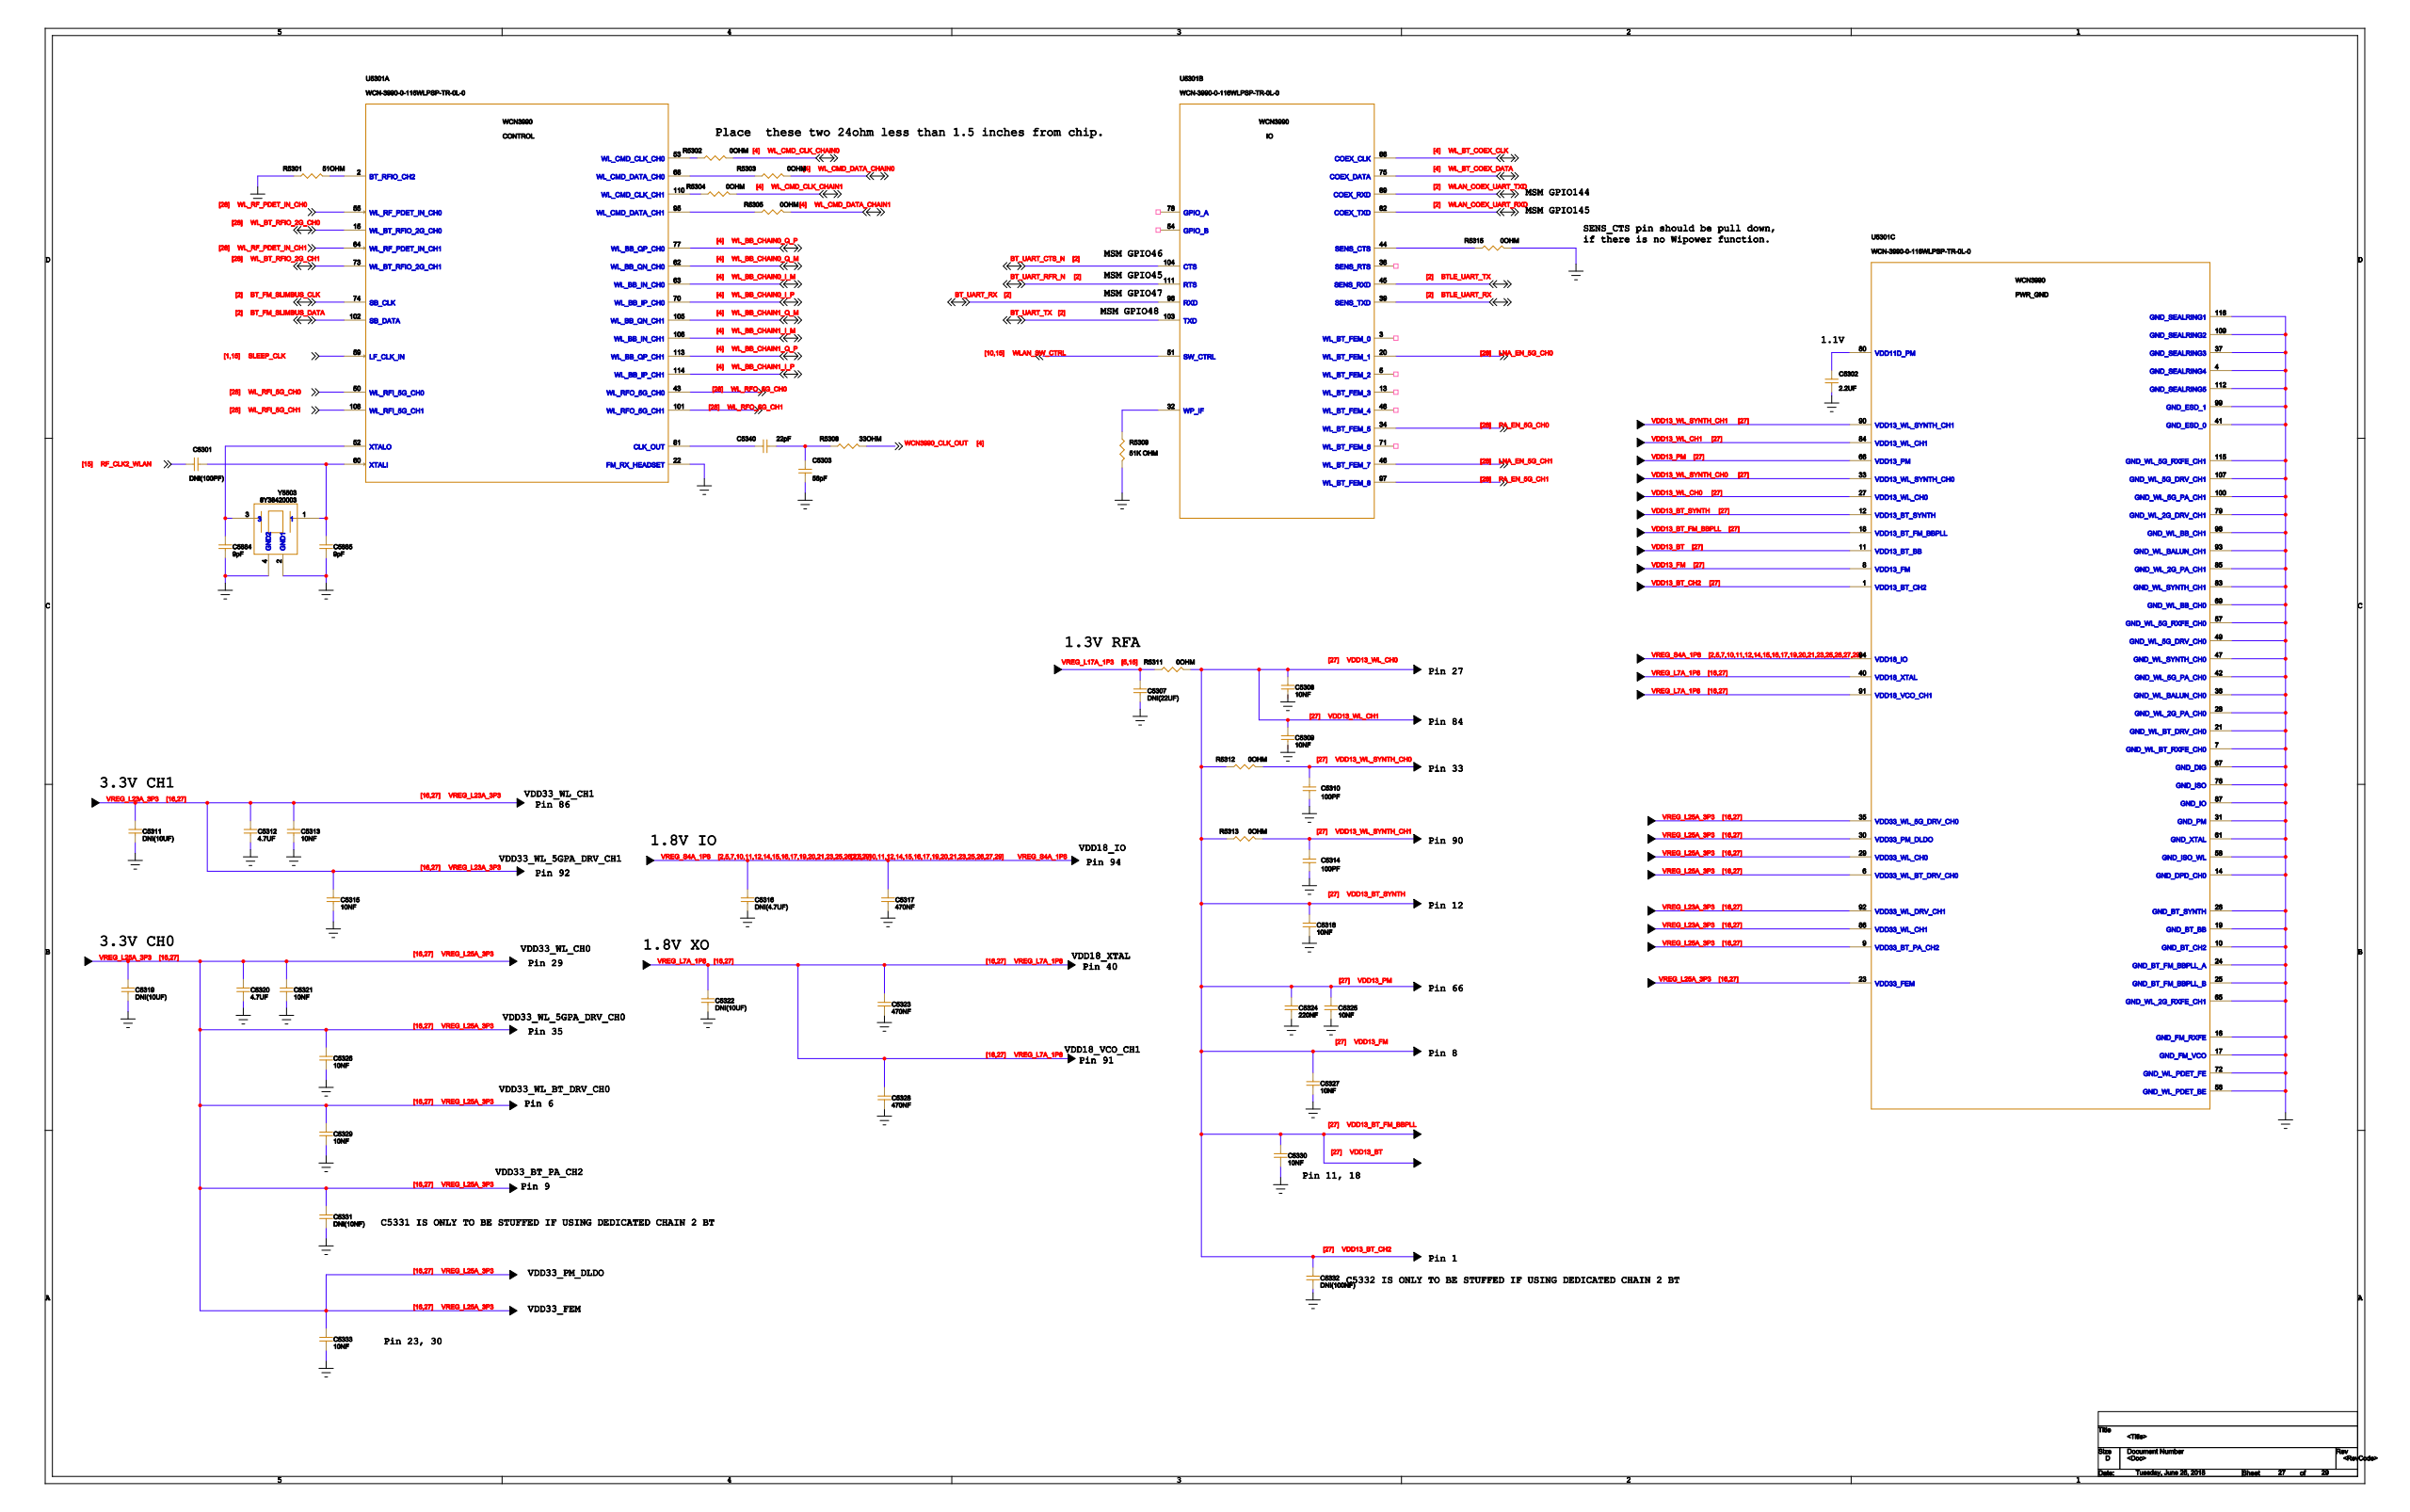Circuit board | Cadence Allegro | 802 parts | 566 nets | one sheet of the schematic
Parts on this sheet (reference | value | footprint):
C5301 | DNI(100pf) | C0201
C5302 | 2.2uF | 0402-BIG
C5303 | 56pF | C0201
C5307 | DNI(22UF) | 0603-BIG
C5308 | 10nF | C0201
C5309 | 10nF | C0201
C5310 | 100pF | C0201
C5311 | DNI(10UF) | 0402-BIG
C5312 | 4.7uF | 0402-BIG
C5313 | 10nF | C0201
C5314 | 100pF | C0201
C5315 | 10nF | C0201
C5316 | DNI(4.7UF) | 0402-BIG
C5317 | 470nF | C0201
C5318 | 10nF | C0201
C5319 | DNI(10UF) | 0402-BIG
C5320 | 4.7uF | 0402-BIG
C5321 | 10nF | C0201
C5322 | DNI(10UF) | 0402-BIG
C5323 | 470nF | C0201
C5324 | 220NF | C0201
C5325 | 10nF | C0201
C5326 | 10nF | C0201
C5327 | 10nF | C0201
C5328 | 470nF | C0201
C5329 | 10nF | C0201
C5330 | 10nF | C0201
C5331 | DNI(10nF) | C0201
C5332 | DNI(100NF) | C0201
C5333 | 10nF | C0201
C5340 | 22pF | C0201
C5884 | 9pF | C0201
C5885 | 9pF | C0201
R5301 | 51OHM | R0201
R5302 | 0OHM | R0201
R5303 | 0OHM | R0201
R5304 | 0OHM | R0201
R5305 | 0OHM | R0201
R5308 | 33OHM | R0201
R5309 | 51K OHM | R0201
R5311 | 0OHM | R0402
R5312 | 0OHM | R0201
R5313 | 0OHM | R0201
R5315 | 0OHM | R0201
U5301 | WCN-3990-0-116WLPSP-TR-0L-0 | WLPSP116_4P07X3P97X0P65_0P35
Y5503 | 8Y38420003 | Y4_8Y40090004
Nets of these parts (net: part-pin ...):
GND: C5302-2 C5303-2 C5307-2 C5308-2 C5309-2 C5310-1 C5311-2 C5312-2 C5313-2 C5314-1 C5315-2 C5316-2 C5317-2 C5318-2 C5319-2 C5320-2 C5321-2 C5322-2 C5323-2 C5324-2 C5325-2 C5326-2 C5327-2 C5328-2 C5329-2 C5330-2 C5331-2 C5332-2 C5333-2 C5884-2 C5885-2 R5301-1 R5309-2 R5315-2 Y5503-2 Y5503-4 U5301-4 U5301-7 U5301-10 U5301-14 U5301-16 U5301-17 U5301-19 U5301-21 U5301-22 U5301-24 U5301-25 U5301-26 U5301-28 U5301-31 U5301-36 U5301-37 U5301-41 U5301-42 U5301-47 U5301-49 U5301-56 U5301-57 U5301-58 U5301-61 U5301-65 U5301-67 U5301-69 U5301-72 U5301-76 U5301-79 U5301-83 U5301-85 U5301-87 U5301-93 U5301-98 U5301-99 U5301-100 U5301-107 U5301-109 U5301-112 U5301-115 U5301-116
VREG_L25A_3P3: C5319-1 C5320-1 C5321-1 C5326-1 C5329-1 C5331-1 C5333-1 U5301-6 U5301-9 U5301-23 U5301-29 U5301-30 U5301-35
WL_RFO_5G_CH0: U5301-43
WL_RFO_5G_CH1: U5301-101
VREG_S4A_1P8: C5316-1 C5317-1 U5301-94
RF_CLK2_WLAN: C5301-1
N1101497: C5301-2 C5885-1 Y5503-1 U5301-60
VREG_L7A_1P8: C5322-1 C5323-1 C5328-1 U5301-40 U5301-91
VDD13_WL_SYNTH_CH0: C5310-2 R5312-2 U5301-33
VDD13_WL_SYNTH_CH1: C5314-2 R5313-2 U5301-90
VREG_L17A_1P3: C5307-1 R5311-1
WL_RF_PDET_IN_CH0: U5301-55
WL_RF_PDET_IN_CH1: U5301-64
VDD13_BT: C5308-1 C5309-1 C5318-1 C5324-1 C5325-1 C5327-1 C5330-1 C5332-1 R5311-2 R5312-1 R5313-1 U5301-1 U5301-8 U5301-11 U5301-12 U5301-18 U5301-27 U5301-66 U5301-84
N1102137: C5302-1 U5301-80
VREG_L23A_3P3: C5311-1 C5312-1 C5313-1 C5315-1 U5301-86 U5301-92
N1101605: C5303-1 C5340-2 R5308-1
N1101601: C5340-1 U5301-81
LNA_EN_5G_CH0: U5301-20
PA_EN_5G_CH0: U5301-34
PA_EN_5G_CH1: U5301-97
LNA_EN_5G_CH1: U5301-46
WL_BT_RFIO_2G_CH0: U5301-15
WL_BT_RFIO_2G_CH1: U5301-73
N1101537: C5884-1 Y5503-3 U5301-52
BT_FM_SLIMBUS_CLK: U5301-74
N1100849: R5302-1 U5301-53
WL_CMD_CLK_CHAIN0: R5302-2
N1100857: R5303-1 U5301-68
WL_CMD_DATA_CHAIN0: R5303-2
N1100853: R5304-1 U5301-110
WL_CMD_CLK_CHAIN1: R5304-2
N1100881: R5305-1 U5301-95
WL_CMD_DATA_CHAIN1: R5305-2
N1101911: R5315-1 U5301-44
N1100593: R5301-2 U5301-2
WCN3990_CLK_OUT: R5308-2
N1101763: R5309-1 U5301-32
SLEEP_CLK: U5301-59
BT_UART_RFR_N: U5301-111
BT_UART_CTS_N: U5301-104
BT_UART_RX: U5301-96
BT_UART_TX: U5301-103
BT_FM_SLIMBUS_DATA: U5301-102
WLAN_COEX_UART_TXD: U5301-89
WLAN_COEX_UART_RXD: U5301-82
BTLE_UART_TX: U5301-45
BTLE_UART_RX: U5301-39
WL_BT_COEX_CLK: U5301-88
WL_BT_COEX_DATA: U5301-75
WL_BB_CHAIN0_I_M: U5301-63
WL_BB_CHAIN0_I_P: U5301-70
WL_BB_CHAIN0_Q_M: U5301-62
WL_BB_CHAIN0_Q_P: U5301-77
WL_BB_CHAIN1_I_M: U5301-106
WL_BB_CHAIN1_I_P: U5301-114
WL_BB_CHAIN1_Q_M: U5301-105
WL_BB_CHAIN1_Q_P: U5301-113
WLAN_SW_CTRL: U5301-51
WL_RFI_5G_CH0: U5301-50
WL_RFI_5G_CH1: U5301-108